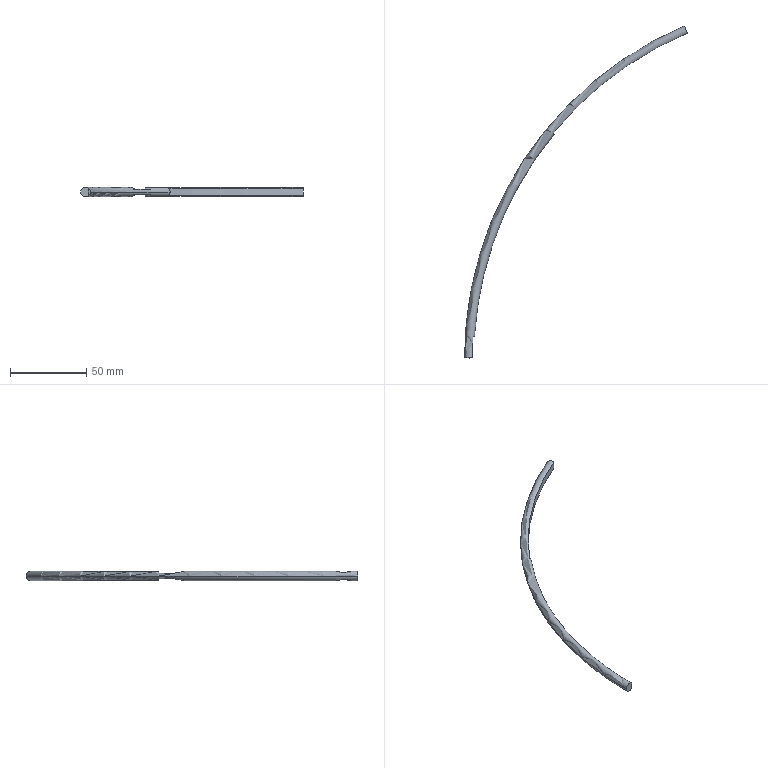Part | SolidWorks | features ICE 1, Sweep 1 | 1 solid | 8 faces | box 145.741 x 217.239 x 6 mm | volume 7317 mm3 | plane 4 | torus 2 | cylinder 2 | commonest cylinder face diameters 462 x2
STEP:
#1=CARTESIAN_POINT('',(-90.259,212.637,2.236));
#2=VERTEX_POINT('',#1);
#3=CARTESIAN_POINT('',(-92.213,217.239,0.));
#4=VERTEX_POINT('',#3);
#5=CARTESIAN_POINT('',(-91.04,214.478,0.));
#6=DIRECTION('',(-0.9205,-0.3907,0.));
#7=DIRECTION('',(0.3907,-0.9205,0.));
#8=AXIS2_PLACEMENT_3D('',#5,#6,#7);
#9=CIRCLE('',#8,3.);
#10=EDGE_CURVE('',#2,#4,#9,.T.);
#11=ORIENTED_EDGE('',*,*,#10,.T.);
#12=CARTESIAN_POINT('',(-236.,0.,0.));
#13=VERTEX_POINT('',#12);
#14=CARTESIAN_POINT('',(0.,0.,0.));
#15=DIRECTION('',(0.,0.,1.));
#16=DIRECTION('',(1.,0.,0.));
#17=AXIS2_PLACEMENT_3D('',#14,#15,#16);
#18=CIRCLE('',#17,236.);
#19=EDGE_CURVE('',#4,#13,#18,.T.);
#20=ORIENTED_EDGE('',*,*,#19,.T.);
#21=CARTESIAN_POINT('',(-231.,0.,2.236));
#22=VERTEX_POINT('',#21);
#23=CARTESIAN_POINT('',(-233.,0.,0.));
#24=DIRECTION('',(0.,-1.,0.));
#25=DIRECTION('',(1.,0.,0.));
#26=AXIS2_PLACEMENT_3D('',#23,#24,#25);
#27=CIRCLE('',#26,3.);
#28=EDGE_CURVE('',#22,#13,#27,.T.);
#29=ORIENTED_EDGE('',*,*,#28,.F.);
#30=CARTESIAN_POINT('',(-230.569,14.102,2.236));
#31=VERTEX_POINT('',#30);
#32=CARTESIAN_POINT('',(0.,0.,2.236));
#33=DIRECTION('',(0.,0.,1.));
#34=DIRECTION('',(-1.,0.,0.));
#35=AXIS2_PLACEMENT_3D('',#32,#33,#34);
#36=CIRCLE('',#35,231.);
#37=EDGE_CURVE('',#31,#22,#36,.T.);
#38=ORIENTED_EDGE('',*,*,#37,.F.);
#39=CARTESIAN_POINT('',(-229.571,14.041,0.));
#40=VERTEX_POINT('',#39);
#41=CARTESIAN_POINT('',(-232.565,14.224,0.));
#42=DIRECTION('',(-0.06105,-0.9981,0.));
#43=DIRECTION('',(-0.9981,0.06105,0.));
#44=AXIS2_PLACEMENT_3D('',#41,#42,#43);
#45=CIRCLE('',#44,3.);
#46=EDGE_CURVE('',#40,#31,#45,.T.);
#47=ORIENTED_EDGE('',*,*,#46,.F.);
#48=CARTESIAN_POINT('',(-177.474,146.298,0.));
#49=VERTEX_POINT('',#48);
#50=CARTESIAN_POINT('',(0.,0.,0.));
#51=DIRECTION('',(0.,0.,1.));
#52=DIRECTION('',(1.,0.,0.));
#53=AXIS2_PLACEMENT_3D('',#50,#51,#52);
#54=CIRCLE('',#53,230.);
#55=EDGE_CURVE('',#49,#40,#54,.T.);
#56=ORIENTED_EDGE('',*,*,#55,.F.);
#57=CARTESIAN_POINT('',(-178.245,146.934,2.236));
#58=VERTEX_POINT('',#57);
#59=CARTESIAN_POINT('',(-179.789,148.206,0.));
#60=DIRECTION('',(-0.6361,-0.7716,0.));
#61=DIRECTION('',(-0.7716,0.6361,0.));
#62=AXIS2_PLACEMENT_3D('',#59,#60,#61);
#63=CIRCLE('',#62,3.);
#64=EDGE_CURVE('',#49,#58,#63,.T.);
#65=ORIENTED_EDGE('',*,*,#64,.T.);
#66=CARTESIAN_POINT('',(0.,0.,2.236));
#67=DIRECTION('',(0.,0.,1.));
#68=DIRECTION('',(-1.,0.,0.));
#69=AXIS2_PLACEMENT_3D('',#66,#67,#68);
#70=CIRCLE('',#69,231.);
#71=EDGE_CURVE('',#2,#58,#70,.T.);
#72=ORIENTED_EDGE('',*,*,#71,.F.);
#73=EDGE_LOOP('',(#11,#20,#29,#38,#47,#56,#65,#72));
#74=FACE_OUTER_BOUND('',#73,.T.);
#75=CARTESIAN_POINT('',(0.,0.,0.));
#76=DIRECTION('',(0.,0.,1.));
#77=DIRECTION('',(1.,0.,0.));
#78=AXIS2_PLACEMENT_3D('',#75,#76,#77);
#79=TOROIDAL_SURFACE('',#78,233.,3.);
#80=ADVANCED_FACE('',(#74),#79,.T.);
#81=ORIENTED_EDGE('',*,*,#19,.F.);
#82=CARTESIAN_POINT('',(-90.259,212.637,-2.236));
#83=VERTEX_POINT('',#82);
#84=CARTESIAN_POINT('',(-91.04,214.478,0.));
#85=DIRECTION('',(-0.9205,-0.3907,0.));
#86=DIRECTION('',(0.3907,-0.9205,0.));
#87=AXIS2_PLACEMENT_3D('',#84,#85,#86);
#88=CIRCLE('',#87,3.);
#89=EDGE_CURVE('',#4,#83,#88,.T.);
#90=ORIENTED_EDGE('',*,*,#89,.T.);
#91=CARTESIAN_POINT('',(-178.245,146.934,-2.236));
#92=VERTEX_POINT('',#91);
#93=CARTESIAN_POINT('',(0.,0.,-2.236));
#94=DIRECTION('',(0.,0.,-1.));
#95=DIRECTION('',(1.,0.,0.));
#96=AXIS2_PLACEMENT_3D('',#93,#94,#95);
#97=CIRCLE('',#96,231.);
#98=EDGE_CURVE('',#92,#83,#97,.T.);
#99=ORIENTED_EDGE('',*,*,#98,.F.);
#100=CARTESIAN_POINT('',(-179.789,148.206,0.));
#101=DIRECTION('',(-0.6361,-0.7716,0.));
#102=DIRECTION('',(-0.7716,0.6361,0.));
#103=AXIS2_PLACEMENT_3D('',#100,#101,#102);
#104=CIRCLE('',#103,3.);
#105=EDGE_CURVE('',#92,#49,#104,.T.);
#106=ORIENTED_EDGE('',*,*,#105,.T.);
#107=ORIENTED_EDGE('',*,*,#55,.T.);
#108=CARTESIAN_POINT('',(-230.569,14.102,-2.236));
#109=VERTEX_POINT('',#108);
#110=CARTESIAN_POINT('',(-232.565,14.224,0.));
#111=DIRECTION('',(-0.06105,-0.9981,0.));
#112=DIRECTION('',(-0.9981,0.06105,0.));
#113=AXIS2_PLACEMENT_3D('',#110,#111,#112);
#114=CIRCLE('',#113,3.);
#115=EDGE_CURVE('',#109,#40,#114,.T.);
#116=ORIENTED_EDGE('',*,*,#115,.F.);
#117=CARTESIAN_POINT('',(-231.,0.,-2.236));
#118=VERTEX_POINT('',#117);
#119=CARTESIAN_POINT('',(0.,0.,-2.236));
#120=DIRECTION('',(0.,0.,-1.));
#121=DIRECTION('',(1.,0.,0.));
#122=AXIS2_PLACEMENT_3D('',#119,#120,#121);
#123=CIRCLE('',#122,231.);
#124=EDGE_CURVE('',#118,#109,#123,.T.);
#125=ORIENTED_EDGE('',*,*,#124,.F.);
#126=CARTESIAN_POINT('',(-233.,0.,0.));
#127=DIRECTION('',(0.,-1.,0.));
#128=DIRECTION('',(1.,0.,0.));
#129=AXIS2_PLACEMENT_3D('',#126,#127,#128);
#130=CIRCLE('',#129,3.);
#131=EDGE_CURVE('',#13,#118,#130,.T.);
#132=ORIENTED_EDGE('',*,*,#131,.F.);
#133=EDGE_LOOP('',(#81,#90,#99,#106,#107,#116,#125,#132));
#134=FACE_OUTER_BOUND('',#133,.T.);
#135=CARTESIAN_POINT('',(0.,0.,0.));
#136=DIRECTION('',(0.,0.,1.));
#137=DIRECTION('',(1.,0.,0.));
#138=AXIS2_PLACEMENT_3D('',#135,#136,#137);
#139=TOROIDAL_SURFACE('',#138,233.,3.);
#140=ADVANCED_FACE('',(#134),#139,.T.);
#141=CARTESIAN_POINT('',(-231.,0.,-25.));
#142=DIRECTION('',(0.,0.,1.));
#143=VECTOR('',#142,1000.);
#144=LINE('',#141,#143);
#145=EDGE_CURVE('',#118,#22,#144,.T.);
#146=ORIENTED_EDGE('',*,*,#145,.T.);
#147=ORIENTED_EDGE('',*,*,#28,.T.);
#148=ORIENTED_EDGE('',*,*,#131,.T.);
#149=EDGE_LOOP('',(#146,#147,#148));
#150=FACE_OUTER_BOUND('',#149,.T.);
#151=CARTESIAN_POINT('',(-233.,0.,0.));
#152=DIRECTION('',(0.,-1.,0.));
#153=DIRECTION('',(1.,0.,0.));
#154=AXIS2_PLACEMENT_3D('',#151,#152,#153);
#155=PLANE('',#154);
#156=ADVANCED_FACE('',(#150),#155,.T.);
#157=ORIENTED_EDGE('',*,*,#10,.F.);
#158=CARTESIAN_POINT('',(-90.259,212.637,-25.));
#159=DIRECTION('',(0.,0.,1.));
#160=VECTOR('',#159,1000.);
#161=LINE('',#158,#160);
#162=EDGE_CURVE('',#83,#2,#161,.T.);
#163=ORIENTED_EDGE('',*,*,#162,.F.);
#164=ORIENTED_EDGE('',*,*,#89,.F.);
#165=EDGE_LOOP('',(#157,#163,#164));
#166=FACE_OUTER_BOUND('',#165,.T.);
#167=CARTESIAN_POINT('',(-91.04,214.478,0.));
#168=DIRECTION('',(-0.9205,-0.3907,0.));
#169=DIRECTION('',(0.3907,-0.9205,0.));
#170=AXIS2_PLACEMENT_3D('',#167,#168,#169);
#171=PLANE('',#170);
#172=ADVANCED_FACE('',(#166),#171,.F.);
#173=ORIENTED_EDGE('',*,*,#115,.T.);
#174=ORIENTED_EDGE('',*,*,#46,.T.);
#175=CARTESIAN_POINT('',(-230.569,14.102,-25.));
#176=DIRECTION('',(0.,0.,1.));
#177=VECTOR('',#176,1000.);
#178=LINE('',#175,#177);
#179=EDGE_CURVE('',#109,#31,#178,.T.);
#180=ORIENTED_EDGE('',*,*,#179,.F.);
#181=EDGE_LOOP('',(#173,#174,#180));
#182=FACE_OUTER_BOUND('',#181,.T.);
#183=CARTESIAN_POINT('',(0.,0.,-25.));
#184=DIRECTION('',(0.06105,0.9981,0.));
#185=DIRECTION('',(-0.9981,0.06105,0.));
#186=AXIS2_PLACEMENT_3D('',#183,#184,#185);
#187=PLANE('',#186);
#188=ADVANCED_FACE('',(#182),#187,.F.);
#189=ORIENTED_EDGE('',*,*,#37,.T.);
#190=ORIENTED_EDGE('',*,*,#145,.F.);
#191=ORIENTED_EDGE('',*,*,#124,.T.);
#192=ORIENTED_EDGE('',*,*,#179,.T.);
#193=EDGE_LOOP('',(#189,#190,#191,#192));
#194=FACE_OUTER_BOUND('',#193,.T.);
#195=CARTESIAN_POINT('',(0.,0.,-25.));
#196=DIRECTION('',(0.,0.,1.));
#197=DIRECTION('',(1.,0.,0.));
#198=AXIS2_PLACEMENT_3D('',#195,#196,#197);
#199=CYLINDRICAL_SURFACE('',#198,231.);
#200=ADVANCED_FACE('',(#194),#199,.F.);
#201=CARTESIAN_POINT('',(-178.245,146.934,-25.));
#202=DIRECTION('',(0.,0.,1.));
#203=VECTOR('',#202,1000.);
#204=LINE('',#201,#203);
#205=EDGE_CURVE('',#92,#58,#204,.T.);
#206=ORIENTED_EDGE('',*,*,#205,.T.);
#207=ORIENTED_EDGE('',*,*,#64,.F.);
#208=ORIENTED_EDGE('',*,*,#105,.F.);
#209=EDGE_LOOP('',(#206,#207,#208));
#210=FACE_OUTER_BOUND('',#209,.T.);
#211=CARTESIAN_POINT('',(0.,0.,-25.));
#212=DIRECTION('',(0.6361,0.7716,0.));
#213=DIRECTION('',(-0.7716,0.6361,0.));
#214=AXIS2_PLACEMENT_3D('',#211,#212,#213);
#215=PLANE('',#214);
#216=ADVANCED_FACE('',(#210),#215,.T.);
#217=ORIENTED_EDGE('',*,*,#71,.T.);
#218=ORIENTED_EDGE('',*,*,#205,.F.);
#219=ORIENTED_EDGE('',*,*,#98,.T.);
#220=ORIENTED_EDGE('',*,*,#162,.T.);
#221=EDGE_LOOP('',(#217,#218,#219,#220));
#222=FACE_OUTER_BOUND('',#221,.T.);
#223=CARTESIAN_POINT('',(0.,0.,-25.));
#224=DIRECTION('',(0.,0.,1.));
#225=DIRECTION('',(1.,0.,0.));
#226=AXIS2_PLACEMENT_3D('',#223,#224,#225);
#227=CYLINDRICAL_SURFACE('',#226,231.);
#228=ADVANCED_FACE('',(#222),#227,.F.);
#229=CLOSED_SHELL('',(#80,#140,#156,#172,#188,#200,#216,#228));
#230=MANIFOLD_SOLID_BREP('',#229);
#231=CARTESIAN_POINT('',(0.,0.,0.));
#232=DIRECTION('',(0.,0.,1.));
#233=DIRECTION('',(1.,0.,0.));
#234=AXIS2_PLACEMENT_3D('',#231,#232,#233);
#235=(LENGTH_UNIT()NAMED_UNIT(*)SI_UNIT(.MILLI.,.METRE.));
#236=UNCERTAINTY_MEASURE_WITH_UNIT(LENGTH_MEASURE(0.00001),#235,'','');
#237=(NAMED_UNIT(*)PLANE_ANGLE_UNIT()SI_UNIT($,.RADIAN.));
#238=(NAMED_UNIT(*)SI_UNIT($,.STERADIAN.)SOLID_ANGLE_UNIT());
#239=(GEOMETRIC_REPRESENTATION_CONTEXT(3)GLOBAL_UNCERTAINTY_ASSIGNED_CONTEXT((#236))GLOBAL_UNIT_ASSIGNED_CONTEXT((#235,#237,#238))REPRESENTATION_CONTEXT('',''));
#240=ADVANCED_BREP_SHAPE_REPRESENTATION('',(#230,#234),#239);